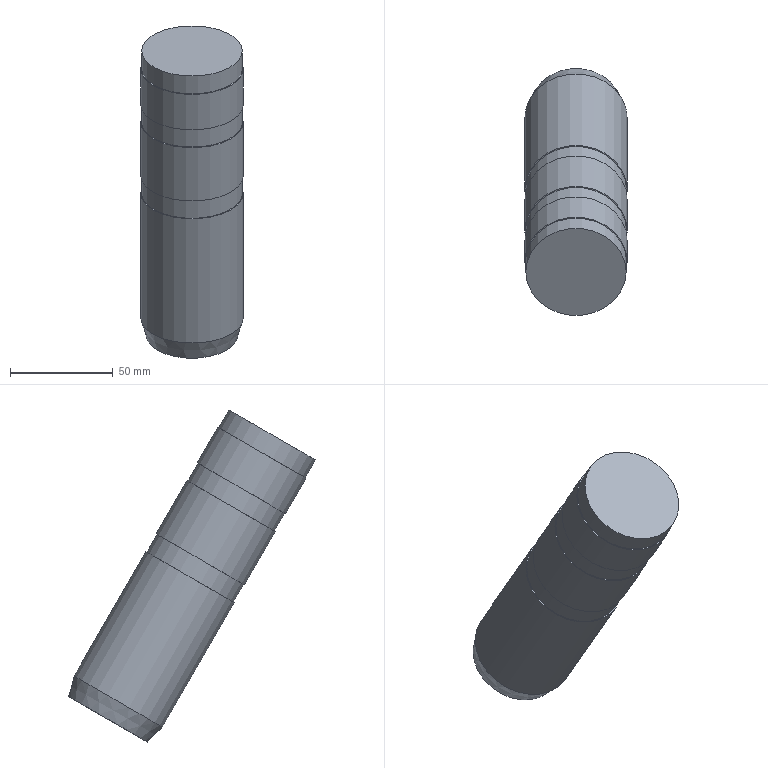Part | NX | features solid 2 | 1 solid | 14 faces | box 50 x 120.548 x 161.974 mm | volume 309797 mm3 | plane 7 | cylinder 6 | cone 1 | commonest cylinder face diameters 49 x3 50 x3
STEP:
#1=CARTESIAN_POINT('',(280.5,-417.513,135.263));
#2=VERTEX_POINT('',#1);
#3=CARTESIAN_POINT('',(305.,-417.513,135.263));
#4=DIRECTION('',(0.,0.5,-0.866));
#5=DIRECTION('',(-1.,0.,0.));
#6=AXIS2_PLACEMENT_3D('',#3,#4,#5);
#7=CIRCLE('',#6,24.5);
#8=EDGE_CURVE('',#2,#2,#7,.T.);
#9=ORIENTED_EDGE('',*,*,#8,.F.);
#10=EDGE_LOOP('',(#9));
#11=FACE_BOUND('',#10,.T.);
#12=CARTESIAN_POINT('',(280.5,-422.513,143.923));
#13=VERTEX_POINT('',#12);
#14=CARTESIAN_POINT('',(305.,-422.513,143.923));
#15=DIRECTION('',(0.,0.5,-0.866));
#16=DIRECTION('',(-1.,0.,0.));
#17=AXIS2_PLACEMENT_3D('',#14,#15,#16);
#18=CIRCLE('',#17,24.5);
#19=EDGE_CURVE('',#13,#13,#18,.T.);
#20=ORIENTED_EDGE('',*,*,#19,.T.);
#21=EDGE_LOOP('',(#20));
#22=FACE_BOUND('',#21,.T.);
#23=CARTESIAN_POINT('',(305.,-417.513,135.263));
#24=DIRECTION('',(0.,-0.5,0.866));
#25=DIRECTION('',(1.,0.,0.));
#26=AXIS2_PLACEMENT_3D('',#23,#24,#25);
#27=CYLINDRICAL_SURFACE('',#26,24.5);
#28=ADVANCED_FACE('',(#11,#22),#27,.T.);
#29=CARTESIAN_POINT('',(280.,-417.513,135.263));
#30=VERTEX_POINT('',#29);
#31=CARTESIAN_POINT('',(305.,-417.513,135.263));
#32=DIRECTION('',(0.,0.5,-0.866));
#33=DIRECTION('',(-1.,0.,0.));
#34=AXIS2_PLACEMENT_3D('',#31,#32,#33);
#35=CIRCLE('',#34,25.);
#36=EDGE_CURVE('',#30,#30,#35,.T.);
#37=ORIENTED_EDGE('',*,*,#36,.F.);
#38=EDGE_LOOP('',(#37));
#39=FACE_BOUND('',#38,.T.);
#40=ORIENTED_EDGE('',*,*,#8,.T.);
#41=EDGE_LOOP('',(#40));
#42=FACE_BOUND('',#41,.T.);
#43=CARTESIAN_POINT('',(305.,-417.513,135.263));
#44=DIRECTION('',(0.,0.5,-0.866));
#45=DIRECTION('',(-1.,0.,0.));
#46=AXIS2_PLACEMENT_3D('',#43,#44,#45);
#47=PLANE('',#46);
#48=ADVANCED_FACE('',(#39,#42),#47,.F.);
#49=CARTESIAN_POINT('',(280.,-382.513,74.641));
#50=VERTEX_POINT('',#49);
#51=CARTESIAN_POINT('',(305.,-382.513,74.641));
#52=DIRECTION('',(0.,0.5,-0.866));
#53=DIRECTION('',(-1.,0.,0.));
#54=AXIS2_PLACEMENT_3D('',#51,#52,#53);
#55=CIRCLE('',#54,25.);
#56=EDGE_CURVE('',#50,#50,#55,.T.);
#57=ORIENTED_EDGE('',*,*,#56,.F.);
#58=EDGE_LOOP('',(#57));
#59=FACE_BOUND('',#58,.T.);
#60=ORIENTED_EDGE('',*,*,#36,.T.);
#61=EDGE_LOOP('',(#60));
#62=FACE_BOUND('',#61,.T.);
#63=CARTESIAN_POINT('',(305.,-382.513,74.641));
#64=DIRECTION('',(0.,-0.5,0.866));
#65=DIRECTION('',(1.,0.,0.));
#66=AXIS2_PLACEMENT_3D('',#63,#64,#65);
#67=CYLINDRICAL_SURFACE('',#66,25.);
#68=ADVANCED_FACE('',(#59,#62),#67,.T.);
#69=CARTESIAN_POINT('',(282.679,-377.513,65.981));
#70=VERTEX_POINT('',#69);
#71=CARTESIAN_POINT('',(305.,-377.513,65.981));
#72=DIRECTION('',(0.,0.5,-0.866));
#73=DIRECTION('',(-1.,0.,0.));
#74=AXIS2_PLACEMENT_3D('',#71,#72,#73);
#75=CIRCLE('',#74,22.321);
#76=EDGE_CURVE('',#70,#70,#75,.T.);
#77=ORIENTED_EDGE('',*,*,#76,.F.);
#78=EDGE_LOOP('',(#77));
#79=FACE_BOUND('',#78,.T.);
#80=ORIENTED_EDGE('',*,*,#56,.T.);
#81=EDGE_LOOP('',(#80));
#82=FACE_BOUND('',#81,.T.);
#83=CARTESIAN_POINT('',(305.,-382.513,74.641));
#84=DIRECTION('',(0.,-0.5,0.866));
#85=DIRECTION('',(-1.,0.,0.));
#86=AXIS2_PLACEMENT_3D('',#83,#84,#85);
#87=CONICAL_SURFACE('',#86,25.,0.2618);
#88=ADVANCED_FACE('',(#79,#82),#87,.T.);
#89=ORIENTED_EDGE('',*,*,#76,.T.);
#90=EDGE_LOOP('',(#89));
#91=FACE_BOUND('',#90,.T.);
#92=CARTESIAN_POINT('',(305.,-377.513,65.981));
#93=DIRECTION('',(0.,0.5,-0.866));
#94=DIRECTION('',(-1.,0.,0.));
#95=AXIS2_PLACEMENT_3D('',#92,#93,#94);
#96=PLANE('',#95);
#97=ADVANCED_FACE('',(#91),#96,.T.);
#98=CARTESIAN_POINT('',(280.,-422.513,143.923));
#99=VERTEX_POINT('',#98);
#100=CARTESIAN_POINT('',(305.,-422.513,143.923));
#101=DIRECTION('',(0.,0.5,-0.866));
#102=DIRECTION('',(-1.,0.,0.));
#103=AXIS2_PLACEMENT_3D('',#100,#101,#102);
#104=CIRCLE('',#103,25.);
#105=EDGE_CURVE('',#99,#99,#104,.T.);
#106=ORIENTED_EDGE('',*,*,#105,.T.);
#107=EDGE_LOOP('',(#106));
#108=FACE_BOUND('',#107,.T.);
#109=ORIENTED_EDGE('',*,*,#19,.F.);
#110=EDGE_LOOP('',(#109));
#111=FACE_BOUND('',#110,.T.);
#112=CARTESIAN_POINT('',(305.,-422.513,143.923));
#113=DIRECTION('',(0.,0.5,-0.866));
#114=DIRECTION('',(-1.,0.,0.));
#115=AXIS2_PLACEMENT_3D('',#112,#113,#114);
#116=PLANE('',#115);
#117=ADVANCED_FACE('',(#108,#111),#116,.T.);
#118=CARTESIAN_POINT('',(280.,-437.513,169.904));
#119=VERTEX_POINT('',#118);
#120=CARTESIAN_POINT('',(305.,-437.513,169.904));
#121=DIRECTION('',(0.,0.5,-0.866));
#122=DIRECTION('',(-1.,0.,0.));
#123=AXIS2_PLACEMENT_3D('',#120,#121,#122);
#124=CIRCLE('',#123,25.);
#125=EDGE_CURVE('',#119,#119,#124,.T.);
#126=ORIENTED_EDGE('',*,*,#125,.T.);
#127=EDGE_LOOP('',(#126));
#128=FACE_BOUND('',#127,.T.);
#129=ORIENTED_EDGE('',*,*,#105,.F.);
#130=EDGE_LOOP('',(#129));
#131=FACE_BOUND('',#130,.T.);
#132=CARTESIAN_POINT('',(305.,-437.513,169.904));
#133=DIRECTION('',(0.,0.5,-0.866));
#134=DIRECTION('',(-1.,0.,0.));
#135=AXIS2_PLACEMENT_3D('',#132,#133,#134);
#136=CYLINDRICAL_SURFACE('',#135,25.);
#137=ADVANCED_FACE('',(#128,#131),#136,.T.);
#138=CARTESIAN_POINT('',(280.5,-437.513,169.904));
#139=VERTEX_POINT('',#138);
#140=CARTESIAN_POINT('',(305.,-437.513,169.904));
#141=DIRECTION('',(0.,0.5,-0.866));
#142=DIRECTION('',(-1.,0.,0.));
#143=AXIS2_PLACEMENT_3D('',#140,#141,#142);
#144=CIRCLE('',#143,24.5);
#145=EDGE_CURVE('',#139,#139,#144,.T.);
#146=ORIENTED_EDGE('',*,*,#145,.T.);
#147=EDGE_LOOP('',(#146));
#148=FACE_BOUND('',#147,.T.);
#149=ORIENTED_EDGE('',*,*,#125,.F.);
#150=EDGE_LOOP('',(#149));
#151=FACE_BOUND('',#150,.T.);
#152=CARTESIAN_POINT('',(305.,-437.513,169.904));
#153=DIRECTION('',(0.,0.5,-0.866));
#154=DIRECTION('',(-1.,0.,0.));
#155=AXIS2_PLACEMENT_3D('',#152,#153,#154);
#156=PLANE('',#155);
#157=ADVANCED_FACE('',(#148,#151),#156,.F.);
#158=CARTESIAN_POINT('',(280.5,-442.513,178.564));
#159=VERTEX_POINT('',#158);
#160=CARTESIAN_POINT('',(305.,-442.513,178.564));
#161=DIRECTION('',(0.,0.5,-0.866));
#162=DIRECTION('',(-1.,0.,0.));
#163=AXIS2_PLACEMENT_3D('',#160,#161,#162);
#164=CIRCLE('',#163,24.5);
#165=EDGE_CURVE('',#159,#159,#164,.F.);
#166=ORIENTED_EDGE('',*,*,#165,.F.);
#167=EDGE_LOOP('',(#166));
#168=FACE_BOUND('',#167,.T.);
#169=ORIENTED_EDGE('',*,*,#145,.F.);
#170=EDGE_LOOP('',(#169));
#171=FACE_BOUND('',#170,.T.);
#172=CARTESIAN_POINT('',(305.,-442.513,178.564));
#173=DIRECTION('',(0.,0.5,-0.866));
#174=DIRECTION('',(-1.,0.,0.));
#175=AXIS2_PLACEMENT_3D('',#172,#173,#174);
#176=CYLINDRICAL_SURFACE('',#175,24.5);
#177=ADVANCED_FACE('',(#168,#171),#176,.T.);
#178=CARTESIAN_POINT('',(280.,-452.513,195.885));
#179=VERTEX_POINT('',#178);
#180=CARTESIAN_POINT('',(305.,-452.513,195.885));
#181=DIRECTION('',(0.,0.5,-0.866));
#182=DIRECTION('',(-1.,0.,0.));
#183=AXIS2_PLACEMENT_3D('',#180,#181,#182);
#184=CIRCLE('',#183,25.);
#185=EDGE_CURVE('',#179,#179,#184,.T.);
#186=ORIENTED_EDGE('',*,*,#185,.T.);
#187=EDGE_LOOP('',(#186));
#188=FACE_BOUND('',#187,.T.);
#189=CARTESIAN_POINT('',(280.,-442.513,178.564));
#190=VERTEX_POINT('',#189);
#191=CARTESIAN_POINT('',(305.,-442.513,178.564));
#192=DIRECTION('',(0.,0.5,-0.866));
#193=DIRECTION('',(-1.,0.,0.));
#194=AXIS2_PLACEMENT_3D('',#191,#192,#193);
#195=CIRCLE('',#194,25.);
#196=EDGE_CURVE('',#190,#190,#195,.T.);
#197=ORIENTED_EDGE('',*,*,#196,.F.);
#198=EDGE_LOOP('',(#197));
#199=FACE_BOUND('',#198,.T.);
#200=CARTESIAN_POINT('',(305.,-452.513,195.885));
#201=DIRECTION('',(0.,0.5,-0.866));
#202=DIRECTION('',(-1.,0.,0.));
#203=AXIS2_PLACEMENT_3D('',#200,#201,#202);
#204=CYLINDRICAL_SURFACE('',#203,25.);
#205=ADVANCED_FACE('',(#188,#199),#204,.T.);
#206=CARTESIAN_POINT('',(280.5,-452.513,195.885));
#207=VERTEX_POINT('',#206);
#208=CARTESIAN_POINT('',(305.,-452.513,195.885));
#209=DIRECTION('',(0.,0.5,-0.866));
#210=DIRECTION('',(-1.,0.,0.));
#211=AXIS2_PLACEMENT_3D('',#208,#209,#210);
#212=CIRCLE('',#211,24.5);
#213=EDGE_CURVE('',#207,#207,#212,.T.);
#214=ORIENTED_EDGE('',*,*,#213,.T.);
#215=EDGE_LOOP('',(#214));
#216=FACE_BOUND('',#215,.T.);
#217=ORIENTED_EDGE('',*,*,#185,.F.);
#218=EDGE_LOOP('',(#217));
#219=FACE_BOUND('',#218,.T.);
#220=CARTESIAN_POINT('',(305.,-452.513,195.885));
#221=DIRECTION('',(0.,0.5,-0.866));
#222=DIRECTION('',(-1.,0.,0.));
#223=AXIS2_PLACEMENT_3D('',#220,#221,#222);
#224=PLANE('',#223);
#225=ADVANCED_FACE('',(#216,#219),#224,.F.);
#226=ORIENTED_EDGE('',*,*,#165,.T.);
#227=EDGE_LOOP('',(#226));
#228=FACE_BOUND('',#227,.T.);
#229=ORIENTED_EDGE('',*,*,#196,.T.);
#230=EDGE_LOOP('',(#229));
#231=FACE_BOUND('',#230,.T.);
#232=CARTESIAN_POINT('',(305.,-442.513,178.564));
#233=DIRECTION('',(0.,0.5,-0.866));
#234=DIRECTION('',(-1.,0.,0.));
#235=AXIS2_PLACEMENT_3D('',#232,#233,#234);
#236=PLANE('',#235);
#237=ADVANCED_FACE('',(#228,#231),#236,.T.);
#238=CARTESIAN_POINT('',(280.5,-457.513,204.545));
#239=VERTEX_POINT('',#238);
#240=CARTESIAN_POINT('',(305.,-457.513,204.545));
#241=DIRECTION('',(0.,0.5,-0.866));
#242=DIRECTION('',(-1.,0.,0.));
#243=AXIS2_PLACEMENT_3D('',#240,#241,#242);
#244=CIRCLE('',#243,24.5);
#245=EDGE_CURVE('',#239,#239,#244,.T.);
#246=ORIENTED_EDGE('',*,*,#245,.T.);
#247=EDGE_LOOP('',(#246));
#248=FACE_BOUND('',#247,.T.);
#249=ORIENTED_EDGE('',*,*,#213,.F.);
#250=EDGE_LOOP('',(#249));
#251=FACE_BOUND('',#250,.T.);
#252=CARTESIAN_POINT('',(305.,-457.513,204.545));
#253=DIRECTION('',(0.,0.5,-0.866));
#254=DIRECTION('',(-1.,0.,0.));
#255=AXIS2_PLACEMENT_3D('',#252,#253,#254);
#256=CYLINDRICAL_SURFACE('',#255,24.5);
#257=ADVANCED_FACE('',(#248,#251),#256,.T.);
#258=ORIENTED_EDGE('',*,*,#245,.F.);
#259=EDGE_LOOP('',(#258));
#260=FACE_BOUND('',#259,.T.);
#261=CARTESIAN_POINT('',(305.,-457.513,204.545));
#262=DIRECTION('',(0.,0.5,-0.866));
#263=DIRECTION('',(-1.,0.,0.));
#264=AXIS2_PLACEMENT_3D('',#261,#262,#263);
#265=PLANE('',#264);
#266=ADVANCED_FACE('',(#260),#265,.F.);
#267=CLOSED_SHELL('',(#28,#48,#68,#88,#97,#117,#137,#157,#177,#205,#225,#237,#257,#266));
#268=MANIFOLD_SOLID_BREP('',#267);
#269=(LENGTH_UNIT()NAMED_UNIT(*)SI_UNIT(.MILLI.,.METRE.));
#270=UNCERTAINTY_MEASURE_WITH_UNIT(LENGTH_MEASURE(0.00001),#269,'','');
#271=(NAMED_UNIT(*)PLANE_ANGLE_UNIT()SI_UNIT($,.RADIAN.));
#272=(NAMED_UNIT(*)SI_UNIT($,.STERADIAN.)SOLID_ANGLE_UNIT());
#273=(GEOMETRIC_REPRESENTATION_CONTEXT(3)GLOBAL_UNCERTAINTY_ASSIGNED_CONTEXT((#270))GLOBAL_UNIT_ASSIGNED_CONTEXT((#269,#271,#272))REPRESENTATION_CONTEXT('',''));
#274=ADVANCED_BREP_SHAPE_REPRESENTATION('',(#268),#273);